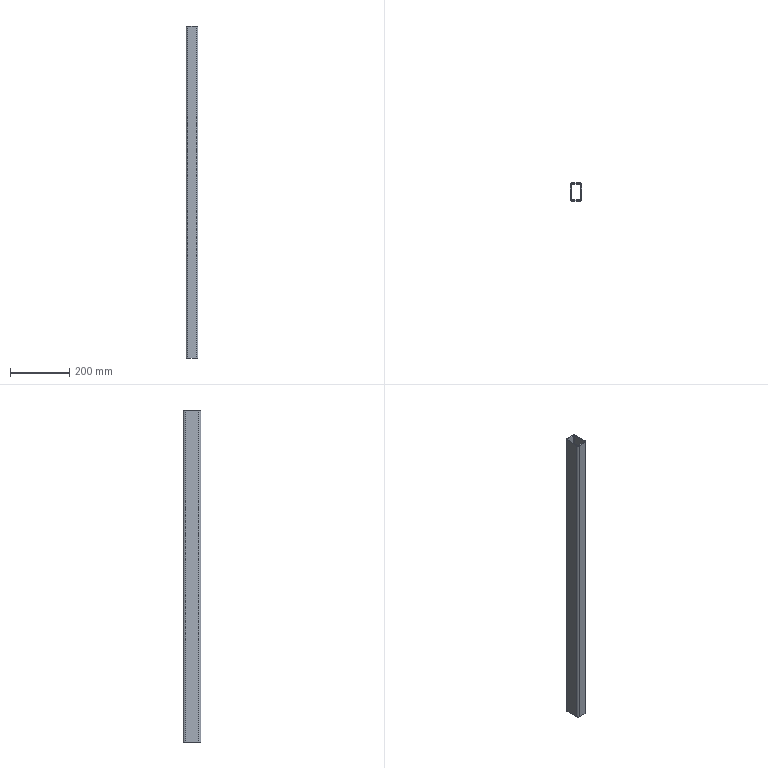Part | STEP file | Profile 40601120 | 1 solid | 18 faces | box 40 x 60 x 1120 mm | volume 641390 mm3 | plane 10 | cylinder 8 | commonest cylinder face diameters 6.4 x4 12.8 x4
STEP:
#1=CARTESIAN_POINT('',(40.,6.4,-600.));
#2=VERTEX_POINT('',#1);
#3=CARTESIAN_POINT('',(40.,6.4,520.));
#4=VERTEX_POINT('',#3);
#5=CARTESIAN_POINT('',(40.,6.4,600.));
#6=DIRECTION('',(0.,0.,1.));
#7=VECTOR('',#6,1000.);
#8=LINE('',#5,#7);
#9=EDGE_CURVE('',#2,#4,#8,.T.);
#10=ORIENTED_EDGE('',*,*,#9,.F.);
#11=CARTESIAN_POINT('',(40.,53.6,-600.));
#12=VERTEX_POINT('',#11);
#13=CARTESIAN_POINT('',(40.,53.6,-600.));
#14=DIRECTION('',(0.,-1.,0.));
#15=VECTOR('',#14,1000.);
#16=LINE('',#13,#15);
#17=EDGE_CURVE('',#12,#2,#16,.T.);
#18=ORIENTED_EDGE('',*,*,#17,.F.);
#19=CARTESIAN_POINT('',(40.,53.6,520.));
#20=VERTEX_POINT('',#19);
#21=CARTESIAN_POINT('',(40.,53.6,600.));
#22=DIRECTION('',(0.,0.,-1.));
#23=VECTOR('',#22,1000.);
#24=LINE('',#21,#23);
#25=EDGE_CURVE('',#20,#12,#24,.T.);
#26=ORIENTED_EDGE('',*,*,#25,.F.);
#27=CARTESIAN_POINT('',(40.,53.6,520.));
#28=DIRECTION('',(0.,1.,0.));
#29=VECTOR('',#28,1000.);
#30=LINE('',#27,#29);
#31=EDGE_CURVE('',#4,#20,#30,.T.);
#32=ORIENTED_EDGE('',*,*,#31,.F.);
#33=EDGE_LOOP('',(#10,#18,#26,#32));
#34=FACE_OUTER_BOUND('',#33,.T.);
#35=CARTESIAN_POINT('',(40.,53.6,600.));
#36=DIRECTION('',(-1.,0.,0.));
#37=DIRECTION('',(0.,0.,1.));
#38=AXIS2_PLACEMENT_3D('',#35,#36,#37);
#39=PLANE('',#38);
#40=ADVANCED_FACE('',(#34),#39,.F.);
#41=CARTESIAN_POINT('',(0.,6.4,520.));
#42=VERTEX_POINT('',#41);
#43=CARTESIAN_POINT('',(6.4,0.,520.));
#44=VERTEX_POINT('',#43);
#45=CARTESIAN_POINT('',(6.4,6.4,520.));
#46=DIRECTION('',(0.,0.,1.));
#47=DIRECTION('',(-1.,0.,0.));
#48=AXIS2_PLACEMENT_3D('',#45,#46,#47);
#49=CIRCLE('',#48,6.4);
#50=EDGE_CURVE('',#42,#44,#49,.T.);
#51=ORIENTED_EDGE('',*,*,#50,.T.);
#52=CARTESIAN_POINT('',(33.6,0.,520.));
#53=VERTEX_POINT('',#52);
#54=CARTESIAN_POINT('',(33.6,0.,520.));
#55=DIRECTION('',(1.,0.,0.));
#56=VECTOR('',#55,1000.);
#57=LINE('',#54,#56);
#58=EDGE_CURVE('',#44,#53,#57,.T.);
#59=ORIENTED_EDGE('',*,*,#58,.T.);
#60=CARTESIAN_POINT('',(33.6,6.4,520.));
#61=DIRECTION('',(0.,0.,1.));
#62=DIRECTION('',(-1.,0.,0.));
#63=AXIS2_PLACEMENT_3D('',#60,#61,#62);
#64=CIRCLE('',#63,6.4);
#65=EDGE_CURVE('',#53,#4,#64,.T.);
#66=ORIENTED_EDGE('',*,*,#65,.T.);
#67=ORIENTED_EDGE('',*,*,#31,.T.);
#68=CARTESIAN_POINT('',(33.6,60.,520.));
#69=VERTEX_POINT('',#68);
#70=CARTESIAN_POINT('',(33.6,53.6,520.));
#71=DIRECTION('',(0.,0.,1.));
#72=DIRECTION('',(-1.,0.,0.));
#73=AXIS2_PLACEMENT_3D('',#70,#71,#72);
#74=CIRCLE('',#73,6.4);
#75=EDGE_CURVE('',#20,#69,#74,.T.);
#76=ORIENTED_EDGE('',*,*,#75,.T.);
#77=CARTESIAN_POINT('',(6.4,60.,520.));
#78=VERTEX_POINT('',#77);
#79=CARTESIAN_POINT('',(33.6,60.,520.));
#80=DIRECTION('',(-1.,0.,0.));
#81=VECTOR('',#80,1000.);
#82=LINE('',#79,#81);
#83=EDGE_CURVE('',#69,#78,#82,.T.);
#84=ORIENTED_EDGE('',*,*,#83,.T.);
#85=CARTESIAN_POINT('',(0.,53.6,520.));
#86=VERTEX_POINT('',#85);
#87=CARTESIAN_POINT('',(6.4,53.6,520.));
#88=DIRECTION('',(0.,0.,1.));
#89=DIRECTION('',(-1.,0.,0.));
#90=AXIS2_PLACEMENT_3D('',#87,#88,#89);
#91=CIRCLE('',#90,6.4);
#92=EDGE_CURVE('',#78,#86,#91,.T.);
#93=ORIENTED_EDGE('',*,*,#92,.T.);
#94=CARTESIAN_POINT('',(0.,6.4,520.));
#95=DIRECTION('',(0.,-1.,0.));
#96=VECTOR('',#95,1000.);
#97=LINE('',#94,#96);
#98=EDGE_CURVE('',#86,#42,#97,.T.);
#99=ORIENTED_EDGE('',*,*,#98,.T.);
#100=EDGE_LOOP('',(#51,#59,#66,#67,#76,#84,#93,#99));
#101=FACE_OUTER_BOUND('',#100,.T.);
#102=CARTESIAN_POINT('',(3.2,53.6,520.));
#103=VERTEX_POINT('',#102);
#104=CARTESIAN_POINT('',(6.4,56.8,520.));
#105=VERTEX_POINT('',#104);
#106=CARTESIAN_POINT('',(6.4,53.6,520.));
#107=DIRECTION('',(0.,0.,-1.));
#108=DIRECTION('',(-1.,0.,0.));
#109=AXIS2_PLACEMENT_3D('',#106,#107,#108);
#110=CIRCLE('',#109,3.2);
#111=EDGE_CURVE('',#103,#105,#110,.T.);
#112=ORIENTED_EDGE('',*,*,#111,.T.);
#113=CARTESIAN_POINT('',(33.6,56.8,520.));
#114=VERTEX_POINT('',#113);
#115=CARTESIAN_POINT('',(33.6,56.8,520.));
#116=DIRECTION('',(1.,0.,0.));
#117=VECTOR('',#116,1000.);
#118=LINE('',#115,#117);
#119=EDGE_CURVE('',#105,#114,#118,.T.);
#120=ORIENTED_EDGE('',*,*,#119,.T.);
#121=CARTESIAN_POINT('',(36.8,53.6,520.));
#122=VERTEX_POINT('',#121);
#123=CARTESIAN_POINT('',(33.6,53.6,520.));
#124=DIRECTION('',(0.,0.,-1.));
#125=DIRECTION('',(-1.,0.,0.));
#126=AXIS2_PLACEMENT_3D('',#123,#124,#125);
#127=CIRCLE('',#126,3.2);
#128=EDGE_CURVE('',#114,#122,#127,.T.);
#129=ORIENTED_EDGE('',*,*,#128,.T.);
#130=CARTESIAN_POINT('',(36.8,6.4,520.));
#131=VERTEX_POINT('',#130);
#132=CARTESIAN_POINT('',(36.8,6.4,520.));
#133=DIRECTION('',(0.,-1.,0.));
#134=VECTOR('',#133,1000.);
#135=LINE('',#132,#134);
#136=EDGE_CURVE('',#122,#131,#135,.T.);
#137=ORIENTED_EDGE('',*,*,#136,.T.);
#138=CARTESIAN_POINT('',(33.6,3.2,520.));
#139=VERTEX_POINT('',#138);
#140=CARTESIAN_POINT('',(33.6,6.4,520.));
#141=DIRECTION('',(0.,0.,-1.));
#142=DIRECTION('',(-1.,0.,0.));
#143=AXIS2_PLACEMENT_3D('',#140,#141,#142);
#144=CIRCLE('',#143,3.2);
#145=EDGE_CURVE('',#131,#139,#144,.T.);
#146=ORIENTED_EDGE('',*,*,#145,.T.);
#147=CARTESIAN_POINT('',(6.4,3.2,520.));
#148=VERTEX_POINT('',#147);
#149=CARTESIAN_POINT('',(33.6,3.2,520.));
#150=DIRECTION('',(-1.,0.,0.));
#151=VECTOR('',#150,1000.);
#152=LINE('',#149,#151);
#153=EDGE_CURVE('',#139,#148,#152,.T.);
#154=ORIENTED_EDGE('',*,*,#153,.T.);
#155=CARTESIAN_POINT('',(3.2,6.4,520.));
#156=VERTEX_POINT('',#155);
#157=CARTESIAN_POINT('',(6.4,6.4,520.));
#158=DIRECTION('',(0.,0.,-1.));
#159=DIRECTION('',(-1.,0.,0.));
#160=AXIS2_PLACEMENT_3D('',#157,#158,#159);
#161=CIRCLE('',#160,3.2);
#162=EDGE_CURVE('',#148,#156,#161,.T.);
#163=ORIENTED_EDGE('',*,*,#162,.T.);
#164=CARTESIAN_POINT('',(3.2,6.4,520.));
#165=DIRECTION('',(0.,1.,0.));
#166=VECTOR('',#165,1000.);
#167=LINE('',#164,#166);
#168=EDGE_CURVE('',#156,#103,#167,.T.);
#169=ORIENTED_EDGE('',*,*,#168,.T.);
#170=EDGE_LOOP('',(#112,#120,#129,#137,#146,#154,#163,#169));
#171=FACE_BOUND('',#170,.T.);
#172=CARTESIAN_POINT('',(33.6,6.4,520.));
#173=DIRECTION('',(0.,0.,1.));
#174=DIRECTION('',(1.,0.,0.));
#175=AXIS2_PLACEMENT_3D('',#172,#173,#174);
#176=PLANE('',#175);
#177=ADVANCED_FACE('',(#101,#171),#176,.T.);
#178=CARTESIAN_POINT('',(33.6,0.,-600.));
#179=VERTEX_POINT('',#178);
#180=CARTESIAN_POINT('',(33.6,0.,600.));
#181=DIRECTION('',(0.,0.,-1.));
#182=VECTOR('',#181,1000.);
#183=LINE('',#180,#182);
#184=EDGE_CURVE('',#53,#179,#183,.T.);
#185=ORIENTED_EDGE('',*,*,#184,.T.);
#186=CARTESIAN_POINT('',(33.6,6.4,-600.));
#187=DIRECTION('',(0.,0.,1.));
#188=DIRECTION('',(-1.,0.,0.));
#189=AXIS2_PLACEMENT_3D('',#186,#187,#188);
#190=CIRCLE('',#189,6.4);
#191=EDGE_CURVE('',#179,#2,#190,.T.);
#192=ORIENTED_EDGE('',*,*,#191,.T.);
#193=ORIENTED_EDGE('',*,*,#9,.T.);
#194=ORIENTED_EDGE('',*,*,#65,.F.);
#195=EDGE_LOOP('',(#185,#192,#193,#194));
#196=FACE_OUTER_BOUND('',#195,.T.);
#197=CARTESIAN_POINT('',(33.6,6.4,600.));
#198=DIRECTION('',(0.,0.,-1.));
#199=DIRECTION('',(-1.,0.,0.));
#200=AXIS2_PLACEMENT_3D('',#197,#198,#199);
#201=CYLINDRICAL_SURFACE('',#200,6.4);
#202=ADVANCED_FACE('',(#196),#201,.T.);
#203=ORIENTED_EDGE('',*,*,#191,.F.);
#204=CARTESIAN_POINT('',(6.4,0.,-600.));
#205=VERTEX_POINT('',#204);
#206=CARTESIAN_POINT('',(33.6,0.,-600.));
#207=DIRECTION('',(1.,0.,0.));
#208=VECTOR('',#207,1000.);
#209=LINE('',#206,#208);
#210=EDGE_CURVE('',#205,#179,#209,.T.);
#211=ORIENTED_EDGE('',*,*,#210,.F.);
#212=CARTESIAN_POINT('',(0.,6.4,-600.));
#213=VERTEX_POINT('',#212);
#214=CARTESIAN_POINT('',(6.4,6.4,-600.));
#215=DIRECTION('',(0.,0.,1.));
#216=DIRECTION('',(-1.,0.,0.));
#217=AXIS2_PLACEMENT_3D('',#214,#215,#216);
#218=CIRCLE('',#217,6.4);
#219=EDGE_CURVE('',#213,#205,#218,.T.);
#220=ORIENTED_EDGE('',*,*,#219,.F.);
#221=CARTESIAN_POINT('',(0.,53.6,-600.));
#222=VERTEX_POINT('',#221);
#223=CARTESIAN_POINT('',(0.,53.6,-600.));
#224=DIRECTION('',(0.,-1.,0.));
#225=VECTOR('',#224,1000.);
#226=LINE('',#223,#225);
#227=EDGE_CURVE('',#222,#213,#226,.T.);
#228=ORIENTED_EDGE('',*,*,#227,.F.);
#229=CARTESIAN_POINT('',(6.4,60.,-600.));
#230=VERTEX_POINT('',#229);
#231=CARTESIAN_POINT('',(6.4,53.6,-600.));
#232=DIRECTION('',(0.,0.,1.));
#233=DIRECTION('',(-1.,0.,0.));
#234=AXIS2_PLACEMENT_3D('',#231,#232,#233);
#235=CIRCLE('',#234,6.4);
#236=EDGE_CURVE('',#230,#222,#235,.T.);
#237=ORIENTED_EDGE('',*,*,#236,.F.);
#238=CARTESIAN_POINT('',(33.6,60.,-600.));
#239=VERTEX_POINT('',#238);
#240=CARTESIAN_POINT('',(33.6,60.,-600.));
#241=DIRECTION('',(-1.,0.,0.));
#242=VECTOR('',#241,1000.);
#243=LINE('',#240,#242);
#244=EDGE_CURVE('',#239,#230,#243,.T.);
#245=ORIENTED_EDGE('',*,*,#244,.F.);
#246=CARTESIAN_POINT('',(33.6,53.6,-600.));
#247=DIRECTION('',(0.,0.,1.));
#248=DIRECTION('',(-1.,0.,0.));
#249=AXIS2_PLACEMENT_3D('',#246,#247,#248);
#250=CIRCLE('',#249,6.4);
#251=EDGE_CURVE('',#12,#239,#250,.T.);
#252=ORIENTED_EDGE('',*,*,#251,.F.);
#253=ORIENTED_EDGE('',*,*,#17,.T.);
#254=EDGE_LOOP('',(#203,#211,#220,#228,#237,#245,#252,#253));
#255=FACE_OUTER_BOUND('',#254,.T.);
#256=CARTESIAN_POINT('',(6.4,3.2,-600.));
#257=VERTEX_POINT('',#256);
#258=CARTESIAN_POINT('',(3.2,6.4,-600.));
#259=VERTEX_POINT('',#258);
#260=CARTESIAN_POINT('',(6.4,6.4,-600.));
#261=DIRECTION('',(0.,0.,-1.));
#262=DIRECTION('',(-1.,0.,0.));
#263=AXIS2_PLACEMENT_3D('',#260,#261,#262);
#264=CIRCLE('',#263,3.2);
#265=EDGE_CURVE('',#257,#259,#264,.T.);
#266=ORIENTED_EDGE('',*,*,#265,.F.);
#267=CARTESIAN_POINT('',(33.6,3.2,-600.));
#268=VERTEX_POINT('',#267);
#269=CARTESIAN_POINT('',(33.6,3.2,-600.));
#270=DIRECTION('',(-1.,0.,0.));
#271=VECTOR('',#270,1000.);
#272=LINE('',#269,#271);
#273=EDGE_CURVE('',#268,#257,#272,.T.);
#274=ORIENTED_EDGE('',*,*,#273,.F.);
#275=CARTESIAN_POINT('',(36.8,6.4,-600.));
#276=VERTEX_POINT('',#275);
#277=CARTESIAN_POINT('',(33.6,6.4,-600.));
#278=DIRECTION('',(0.,0.,-1.));
#279=DIRECTION('',(-1.,0.,0.));
#280=AXIS2_PLACEMENT_3D('',#277,#278,#279);
#281=CIRCLE('',#280,3.2);
#282=EDGE_CURVE('',#276,#268,#281,.T.);
#283=ORIENTED_EDGE('',*,*,#282,.F.);
#284=CARTESIAN_POINT('',(36.8,53.6,-600.));
#285=VERTEX_POINT('',#284);
#286=CARTESIAN_POINT('',(36.8,53.6,-600.));
#287=DIRECTION('',(0.,-1.,0.));
#288=VECTOR('',#287,1000.);
#289=LINE('',#286,#288);
#290=EDGE_CURVE('',#285,#276,#289,.T.);
#291=ORIENTED_EDGE('',*,*,#290,.F.);
#292=CARTESIAN_POINT('',(33.6,56.8,-600.));
#293=VERTEX_POINT('',#292);
#294=CARTESIAN_POINT('',(33.6,53.6,-600.));
#295=DIRECTION('',(0.,0.,-1.));
#296=DIRECTION('',(-1.,0.,0.));
#297=AXIS2_PLACEMENT_3D('',#294,#295,#296);
#298=CIRCLE('',#297,3.2);
#299=EDGE_CURVE('',#293,#285,#298,.T.);
#300=ORIENTED_EDGE('',*,*,#299,.F.);
#301=CARTESIAN_POINT('',(6.4,56.8,-600.));
#302=VERTEX_POINT('',#301);
#303=CARTESIAN_POINT('',(33.6,56.8,-600.));
#304=DIRECTION('',(1.,0.,0.));
#305=VECTOR('',#304,1000.);
#306=LINE('',#303,#305);
#307=EDGE_CURVE('',#302,#293,#306,.T.);
#308=ORIENTED_EDGE('',*,*,#307,.F.);
#309=CARTESIAN_POINT('',(3.2,53.6,-600.));
#310=VERTEX_POINT('',#309);
#311=CARTESIAN_POINT('',(6.4,53.6,-600.));
#312=DIRECTION('',(0.,0.,-1.));
#313=DIRECTION('',(-1.,0.,0.));
#314=AXIS2_PLACEMENT_3D('',#311,#312,#313);
#315=CIRCLE('',#314,3.2);
#316=EDGE_CURVE('',#310,#302,#315,.T.);
#317=ORIENTED_EDGE('',*,*,#316,.F.);
#318=CARTESIAN_POINT('',(3.2,53.6,-600.));
#319=DIRECTION('',(0.,1.,0.));
#320=VECTOR('',#319,1000.);
#321=LINE('',#318,#320);
#322=EDGE_CURVE('',#259,#310,#321,.T.);
#323=ORIENTED_EDGE('',*,*,#322,.F.);
#324=EDGE_LOOP('',(#266,#274,#283,#291,#300,#308,#317,#323));
#325=FACE_BOUND('',#324,.T.);
#326=CARTESIAN_POINT('',(33.6,53.6,-600.));
#327=DIRECTION('',(0.,0.,1.));
#328=DIRECTION('',(1.,0.,0.));
#329=AXIS2_PLACEMENT_3D('',#326,#327,#328);
#330=PLANE('',#329);
#331=ADVANCED_FACE('',(#255,#325),#330,.F.);
#332=ORIENTED_EDGE('',*,*,#25,.T.);
#333=ORIENTED_EDGE('',*,*,#251,.T.);
#334=CARTESIAN_POINT('',(33.6,60.,600.));
#335=DIRECTION('',(0.,0.,1.));
#336=VECTOR('',#335,1000.);
#337=LINE('',#334,#336);
#338=EDGE_CURVE('',#239,#69,#337,.T.);
#339=ORIENTED_EDGE('',*,*,#338,.T.);
#340=ORIENTED_EDGE('',*,*,#75,.F.);
#341=EDGE_LOOP('',(#332,#333,#339,#340));
#342=FACE_OUTER_BOUND('',#341,.T.);
#343=CARTESIAN_POINT('',(33.6,53.6,600.));
#344=DIRECTION('',(0.,0.,-1.));
#345=DIRECTION('',(-1.,0.,0.));
#346=AXIS2_PLACEMENT_3D('',#343,#344,#345);
#347=CYLINDRICAL_SURFACE('',#346,6.4);
#348=ADVANCED_FACE('',(#342),#347,.T.);
#349=CARTESIAN_POINT('',(6.4,0.,600.));
#350=DIRECTION('',(0.,0.,1.));
#351=VECTOR('',#350,1000.);
#352=LINE('',#349,#351);
#353=EDGE_CURVE('',#205,#44,#352,.T.);
#354=ORIENTED_EDGE('',*,*,#353,.F.);
#355=ORIENTED_EDGE('',*,*,#210,.T.);
#356=ORIENTED_EDGE('',*,*,#184,.F.);
#357=ORIENTED_EDGE('',*,*,#58,.F.);
#358=EDGE_LOOP('',(#354,#355,#356,#357));
#359=FACE_OUTER_BOUND('',#358,.T.);
#360=CARTESIAN_POINT('',(6.4,0.,600.));
#361=DIRECTION('',(0.,1.,0.));
#362=DIRECTION('',(-1.,0.,0.));
#363=AXIS2_PLACEMENT_3D('',#360,#361,#362);
#364=PLANE('',#363);
#365=ADVANCED_FACE('',(#359),#364,.F.);
#366=CARTESIAN_POINT('',(0.,6.4,600.));
#367=DIRECTION('',(0.,0.,-1.));
#368=VECTOR('',#367,1000.);
#369=LINE('',#366,#368);
#370=EDGE_CURVE('',#42,#213,#369,.T.);
#371=ORIENTED_EDGE('',*,*,#370,.T.);
#372=ORIENTED_EDGE('',*,*,#219,.T.);
#373=ORIENTED_EDGE('',*,*,#353,.T.);
#374=ORIENTED_EDGE('',*,*,#50,.F.);
#375=EDGE_LOOP('',(#371,#372,#373,#374));
#376=FACE_OUTER_BOUND('',#375,.T.);
#377=CARTESIAN_POINT('',(6.4,6.4,600.));
#378=DIRECTION('',(0.,0.,-1.));
#379=DIRECTION('',(-1.,0.,0.));
#380=AXIS2_PLACEMENT_3D('',#377,#378,#379);
#381=CYLINDRICAL_SURFACE('',#380,6.4);
#382=ADVANCED_FACE('',(#376),#381,.T.);
#383=CARTESIAN_POINT('',(0.,53.6,600.));
#384=DIRECTION('',(0.,0.,1.));
#385=VECTOR('',#384,1000.);
#386=LINE('',#383,#385);
#387=EDGE_CURVE('',#222,#86,#386,.T.);
#388=ORIENTED_EDGE('',*,*,#387,.F.);
#389=ORIENTED_EDGE('',*,*,#227,.T.);
#390=ORIENTED_EDGE('',*,*,#370,.F.);
#391=ORIENTED_EDGE('',*,*,#98,.F.);
#392=EDGE_LOOP('',(#388,#389,#390,#391));
#393=FACE_OUTER_BOUND('',#392,.T.);
#394=CARTESIAN_POINT('',(0.,6.4,600.));
#395=DIRECTION('',(1.,0.,0.));
#396=DIRECTION('',(0.,1.,0.));
#397=AXIS2_PLACEMENT_3D('',#394,#395,#396);
#398=PLANE('',#397);
#399=ADVANCED_FACE('',(#393),#398,.F.);
#400=CARTESIAN_POINT('',(6.4,60.,600.));
#401=DIRECTION('',(0.,0.,-1.));
#402=VECTOR('',#401,1000.);
#403=LINE('',#400,#402);
#404=EDGE_CURVE('',#78,#230,#403,.T.);
#405=ORIENTED_EDGE('',*,*,#404,.T.);
#406=ORIENTED_EDGE('',*,*,#236,.T.);
#407=ORIENTED_EDGE('',*,*,#387,.T.);
#408=ORIENTED_EDGE('',*,*,#92,.F.);
#409=EDGE_LOOP('',(#405,#406,#407,#408));
#410=FACE_OUTER_BOUND('',#409,.T.);
#411=CARTESIAN_POINT('',(6.4,53.6,600.));
#412=DIRECTION('',(0.,0.,-1.));
#413=DIRECTION('',(-1.,0.,0.));
#414=AXIS2_PLACEMENT_3D('',#411,#412,#413);
#415=CYLINDRICAL_SURFACE('',#414,6.4);
#416=ADVANCED_FACE('',(#410),#415,.T.);
#417=ORIENTED_EDGE('',*,*,#338,.F.);
#418=ORIENTED_EDGE('',*,*,#244,.T.);
#419=ORIENTED_EDGE('',*,*,#404,.F.);
#420=ORIENTED_EDGE('',*,*,#83,.F.);
#421=EDGE_LOOP('',(#417,#418,#419,#420));
#422=FACE_OUTER_BOUND('',#421,.T.);
#423=CARTESIAN_POINT('',(33.6,60.,600.));
#424=DIRECTION('',(0.,-1.,0.));
#425=DIRECTION('',(0.,0.,-1.));
#426=AXIS2_PLACEMENT_3D('',#423,#424,#425);
#427=PLANE('',#426);
#428=ADVANCED_FACE('',(#422),#427,.F.);
#429=CARTESIAN_POINT('',(6.4,56.8,600.));
#430=DIRECTION('',(0.,0.,-1.));
#431=VECTOR('',#430,1000.);
#432=LINE('',#429,#431);
#433=EDGE_CURVE('',#105,#302,#432,.T.);
#434=ORIENTED_EDGE('',*,*,#433,.T.);
#435=ORIENTED_EDGE('',*,*,#307,.T.);
#436=CARTESIAN_POINT('',(33.6,56.8,600.));
#437=DIRECTION('',(0.,0.,1.));
#438=VECTOR('',#437,1000.);
#439=LINE('',#436,#438);
#440=EDGE_CURVE('',#293,#114,#439,.T.);
#441=ORIENTED_EDGE('',*,*,#440,.T.);
#442=ORIENTED_EDGE('',*,*,#119,.F.);
#443=EDGE_LOOP('',(#434,#435,#441,#442));
#444=FACE_OUTER_BOUND('',#443,.T.);
#445=CARTESIAN_POINT('',(33.6,56.8,600.));
#446=DIRECTION('',(0.,-1.,0.));
#447=DIRECTION('',(0.,0.,-1.));
#448=AXIS2_PLACEMENT_3D('',#445,#446,#447);
#449=PLANE('',#448);
#450=ADVANCED_FACE('',(#444),#449,.T.);
#451=CARTESIAN_POINT('',(3.2,53.6,600.));
#452=DIRECTION('',(0.,0.,1.));
#453=VECTOR('',#452,1000.);
#454=LINE('',#451,#453);
#455=EDGE_CURVE('',#310,#103,#454,.T.);
#456=ORIENTED_EDGE('',*,*,#455,.F.);
#457=ORIENTED_EDGE('',*,*,#316,.T.);
#458=ORIENTED_EDGE('',*,*,#433,.F.);
#459=ORIENTED_EDGE('',*,*,#111,.F.);
#460=EDGE_LOOP('',(#456,#457,#458,#459));
#461=FACE_OUTER_BOUND('',#460,.T.);
#462=CARTESIAN_POINT('',(6.4,53.6,600.));
#463=DIRECTION('',(0.,0.,-1.));
#464=DIRECTION('',(-1.,0.,0.));
#465=AXIS2_PLACEMENT_3D('',#462,#463,#464);
#466=CYLINDRICAL_SURFACE('',#465,3.2);
#467=ADVANCED_FACE('',(#461),#466,.F.);
#468=CARTESIAN_POINT('',(3.2,6.4,600.));
#469=DIRECTION('',(0.,0.,-1.));
#470=VECTOR('',#469,1000.);
#471=LINE('',#468,#470);
#472=EDGE_CURVE('',#156,#259,#471,.T.);
#473=ORIENTED_EDGE('',*,*,#472,.T.);
#474=ORIENTED_EDGE('',*,*,#322,.T.);
#475=ORIENTED_EDGE('',*,*,#455,.T.);
#476=ORIENTED_EDGE('',*,*,#168,.F.);
#477=EDGE_LOOP('',(#473,#474,#475,#476));
#478=FACE_OUTER_BOUND('',#477,.T.);
#479=CARTESIAN_POINT('',(3.2,6.4,600.));
#480=DIRECTION('',(1.,0.,0.));
#481=DIRECTION('',(0.,1.,0.));
#482=AXIS2_PLACEMENT_3D('',#479,#480,#481);
#483=PLANE('',#482);
#484=ADVANCED_FACE('',(#478),#483,.T.);
#485=CARTESIAN_POINT('',(6.4,3.2,600.));
#486=DIRECTION('',(0.,0.,1.));
#487=VECTOR('',#486,1000.);
#488=LINE('',#485,#487);
#489=EDGE_CURVE('',#257,#148,#488,.T.);
#490=ORIENTED_EDGE('',*,*,#489,.F.);
#491=ORIENTED_EDGE('',*,*,#265,.T.);
#492=ORIENTED_EDGE('',*,*,#472,.F.);
#493=ORIENTED_EDGE('',*,*,#162,.F.);
#494=EDGE_LOOP('',(#490,#491,#492,#493));
#495=FACE_OUTER_BOUND('',#494,.T.);
#496=CARTESIAN_POINT('',(6.4,6.4,600.));
#497=DIRECTION('',(0.,0.,-1.));
#498=DIRECTION('',(-1.,0.,0.));
#499=AXIS2_PLACEMENT_3D('',#496,#497,#498);
#500=CYLINDRICAL_SURFACE('',#499,3.2);
#501=ADVANCED_FACE('',(#495),#500,.F.);
#502=CARTESIAN_POINT('',(33.6,3.2,600.));
#503=DIRECTION('',(0.,0.,-1.));
#504=VECTOR('',#503,1000.);
#505=LINE('',#502,#504);
#506=EDGE_CURVE('',#139,#268,#505,.T.);
#507=ORIENTED_EDGE('',*,*,#506,.T.);
#508=ORIENTED_EDGE('',*,*,#273,.T.);
#509=ORIENTED_EDGE('',*,*,#489,.T.);
#510=ORIENTED_EDGE('',*,*,#153,.F.);
#511=EDGE_LOOP('',(#507,#508,#509,#510));
#512=FACE_OUTER_BOUND('',#511,.T.);
#513=CARTESIAN_POINT('',(6.4,3.2,600.));
#514=DIRECTION('',(0.,1.,0.));
#515=DIRECTION('',(-1.,0.,0.));
#516=AXIS2_PLACEMENT_3D('',#513,#514,#515);
#517=PLANE('',#516);
#518=ADVANCED_FACE('',(#512),#517,.T.);
#519=CARTESIAN_POINT('',(36.8,6.4,600.));
#520=DIRECTION('',(0.,0.,1.));
#521=VECTOR('',#520,1000.);
#522=LINE('',#519,#521);
#523=EDGE_CURVE('',#276,#131,#522,.T.);
#524=ORIENTED_EDGE('',*,*,#523,.F.);
#525=ORIENTED_EDGE('',*,*,#282,.T.);
#526=ORIENTED_EDGE('',*,*,#506,.F.);
#527=ORIENTED_EDGE('',*,*,#145,.F.);
#528=EDGE_LOOP('',(#524,#525,#526,#527));
#529=FACE_OUTER_BOUND('',#528,.T.);
#530=CARTESIAN_POINT('',(33.6,6.4,600.));
#531=DIRECTION('',(0.,0.,-1.));
#532=DIRECTION('',(-1.,0.,0.));
#533=AXIS2_PLACEMENT_3D('',#530,#531,#532);
#534=CYLINDRICAL_SURFACE('',#533,3.2);
#535=ADVANCED_FACE('',(#529),#534,.F.);
#536=CARTESIAN_POINT('',(36.8,53.6,600.));
#537=DIRECTION('',(0.,0.,-1.));
#538=VECTOR('',#537,1000.);
#539=LINE('',#536,#538);
#540=EDGE_CURVE('',#122,#285,#539,.T.);
#541=ORIENTED_EDGE('',*,*,#540,.T.);
#542=ORIENTED_EDGE('',*,*,#290,.T.);
#543=ORIENTED_EDGE('',*,*,#523,.T.);
#544=ORIENTED_EDGE('',*,*,#136,.F.);
#545=EDGE_LOOP('',(#541,#542,#543,#544));
#546=FACE_OUTER_BOUND('',#545,.T.);
#547=CARTESIAN_POINT('',(36.8,53.6,600.));
#548=DIRECTION('',(-1.,0.,0.));
#549=DIRECTION('',(0.,0.,1.));
#550=AXIS2_PLACEMENT_3D('',#547,#548,#549);
#551=PLANE('',#550);
#552=ADVANCED_FACE('',(#546),#551,.T.);
#553=ORIENTED_EDGE('',*,*,#440,.F.);
#554=ORIENTED_EDGE('',*,*,#299,.T.);
#555=ORIENTED_EDGE('',*,*,#540,.F.);
#556=ORIENTED_EDGE('',*,*,#128,.F.);
#557=EDGE_LOOP('',(#553,#554,#555,#556));
#558=FACE_OUTER_BOUND('',#557,.T.);
#559=CARTESIAN_POINT('',(33.6,53.6,600.));
#560=DIRECTION('',(0.,0.,-1.));
#561=DIRECTION('',(-1.,0.,0.));
#562=AXIS2_PLACEMENT_3D('',#559,#560,#561);
#563=CYLINDRICAL_SURFACE('',#562,3.2);
#564=ADVANCED_FACE('',(#558),#563,.F.);
#565=CLOSED_SHELL('',(#40,#177,#202,#331,#348,#365,#382,#399,#416,#428,#450,#467,#484,#501,#518,#535,#552,#564));
#566=MANIFOLD_SOLID_BREP('',#565);
#567=CARTESIAN_POINT('',(0.,0.,0.));
#568=DIRECTION('',(0.,0.,1.));
#569=DIRECTION('',(1.,0.,0.));
#570=AXIS2_PLACEMENT_3D('',#567,#568,#569);
#571=(LENGTH_UNIT()NAMED_UNIT(*)SI_UNIT(.MILLI.,.METRE.));
#572=UNCERTAINTY_MEASURE_WITH_UNIT(LENGTH_MEASURE(0.00001),#571,'','');
#573=(NAMED_UNIT(*)PLANE_ANGLE_UNIT()SI_UNIT($,.RADIAN.));
#574=(NAMED_UNIT(*)SI_UNIT($,.STERADIAN.)SOLID_ANGLE_UNIT());
#575=(GEOMETRIC_REPRESENTATION_CONTEXT(3)GLOBAL_UNCERTAINTY_ASSIGNED_CONTEXT((#572))GLOBAL_UNIT_ASSIGNED_CONTEXT((#571,#573,#574))REPRESENTATION_CONTEXT('',''));
#576=ADVANCED_BREP_SHAPE_REPRESENTATION('',(#566,#570),#575);